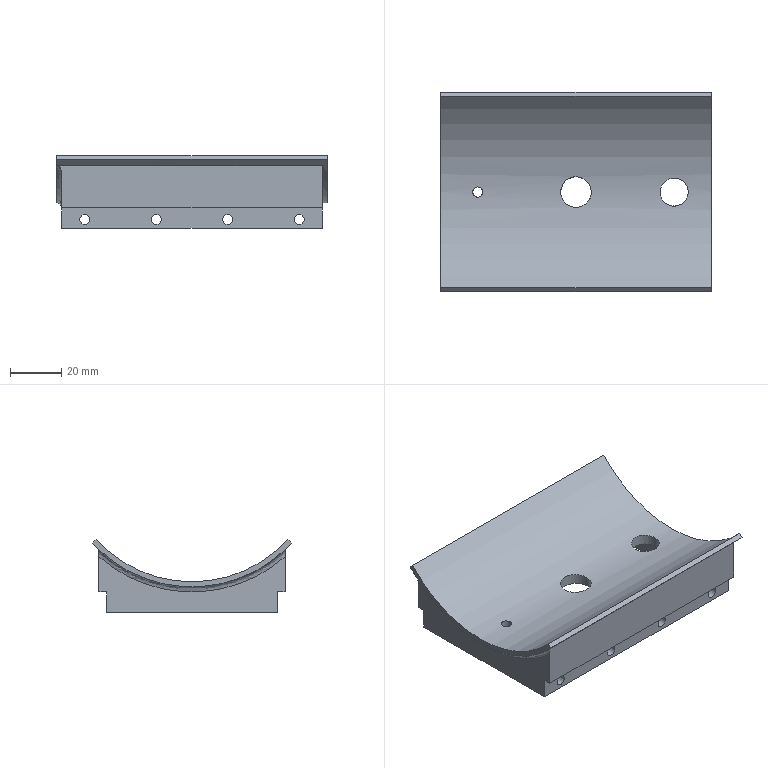Part | STEP file | 1-05 | 1 solid | 32 faces | box 106 x 78.066 x 28.5 mm | volume 78441 mm3 | plane 18 | cylinder 13 | spline 1 | commonest cylinder face diameters 4 x9 11 x1 12 x1 102 x1 106 x1